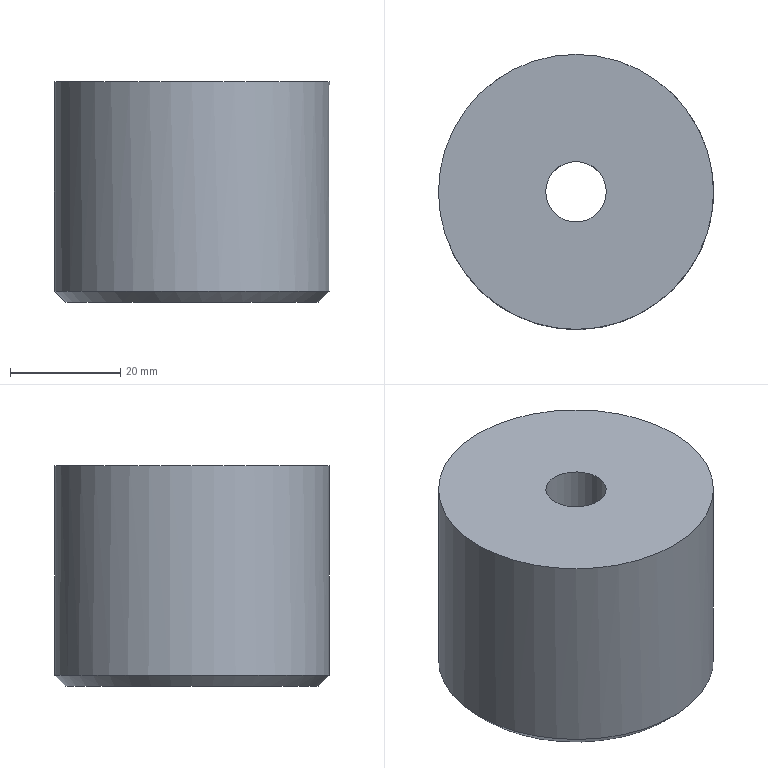Part | STEP file | gslz 2016.10.28-10_id2458_x_t | 1 solid | 7 faces | box 50 x 50 x 40 mm | volume 71266 mm3 | plane 3 | cylinder 3 | cone 1 | commonest cylinder face diameters 11 x1 17 x1 50 x1
STEP:
#1=CARTESIAN_POINT('',(0.,0.,0.));
#2=DIRECTION('',(0.,0.,1.));
#3=DIRECTION('',(1.,0.,0.));
#4=AXIS2_PLACEMENT_3D('',#1,#2,#3);
#5=CARTESIAN_POINT('',(734.,-225.,105.));
#6=VERTEX_POINT('',#5);
#7=CARTESIAN_POINT('',(723.,-225.,105.));
#8=VERTEX_POINT('',#7);
#9=CARTESIAN_POINT('',(728.5,-225.,105.));
#10=DIRECTION('',(0.,0.,1.));
#11=DIRECTION('',(1.,0.,0.));
#12=AXIS2_PLACEMENT_3D('',#9,#10,#11);
#13=CIRCLE('',#12,5.5);
#14=CARTESIAN_POINT('',(676.389,263.723,105.));
#15=DIRECTION('',(0.,0.,1.));
#16=DIRECTION('',(-1.,0.,0.));
#17=AXIS2_PLACEMENT_3D('',#14,#15,#16);
#18=PLANE('',#17);
#19=CARTESIAN_POINT('',(-52.111,488.723));
#20=DIRECTION('',(-1.,0.));
#21=AXIS2_PLACEMENT_2D('',#19,#20);
#22=CIRCLE('',#21,5.5);
#23=(GEOMETRIC_REPRESENTATION_CONTEXT(2)PARAMETRIC_REPRESENTATION_CONTEXT()REPRESENTATION_CONTEXT('',''));
#24=DEFINITIONAL_REPRESENTATION('',(#22),#23);
#25=PCURVE('',#18,#24);
#26=CARTESIAN_POINT('',(728.5,-225.,37.));
#27=DIRECTION('',(0.,0.,1.));
#28=DIRECTION('',(-1.,0.,0.));
#29=AXIS2_PLACEMENT_3D('',#26,#27,#28);
#30=CYLINDRICAL_SURFACE('',#29,5.5);
#31=CARTESIAN_POINT('',(3.142,68.));
#32=DIRECTION('',(1.,0.));
#33=VECTOR('',#32,1.);
#34=LINE('',#31,#33);
#35=(GEOMETRIC_REPRESENTATION_CONTEXT(2)PARAMETRIC_REPRESENTATION_CONTEXT()REPRESENTATION_CONTEXT('',''));
#36=DEFINITIONAL_REPRESENTATION('',(#34),#35);
#37=PCURVE('',#30,#36);
#38=SURFACE_CURVE('',#13,(#25,#37),.PCURVE_S1.);
#39=EDGE_CURVE('',#6,#8,#38,.T.);
#40=ORIENTED_EDGE('',*,*,#39,.F.);
#41=CARTESIAN_POINT('',(728.5,-225.,105.));
#42=DIRECTION('',(0.,0.,1.));
#43=DIRECTION('',(1.,0.,0.));
#44=AXIS2_PLACEMENT_3D('',#41,#42,#43);
#45=CIRCLE('',#44,5.5);
#46=CARTESIAN_POINT('',(-52.111,488.723));
#47=DIRECTION('',(-1.,0.));
#48=AXIS2_PLACEMENT_2D('',#46,#47);
#49=CIRCLE('',#48,5.5);
#50=(GEOMETRIC_REPRESENTATION_CONTEXT(2)PARAMETRIC_REPRESENTATION_CONTEXT()REPRESENTATION_CONTEXT('',''));
#51=DEFINITIONAL_REPRESENTATION('',(#49),#50);
#52=PCURVE('',#18,#51);
#53=CARTESIAN_POINT('',(-3.142,68.));
#54=DIRECTION('',(1.,0.));
#55=VECTOR('',#54,1.);
#56=LINE('',#53,#55);
#57=(GEOMETRIC_REPRESENTATION_CONTEXT(2)PARAMETRIC_REPRESENTATION_CONTEXT()REPRESENTATION_CONTEXT('',''));
#58=DEFINITIONAL_REPRESENTATION('',(#56),#57);
#59=PCURVE('',#30,#58);
#60=SURFACE_CURVE('',#45,(#52,#59),.PCURVE_S1.);
#61=EDGE_CURVE('',#8,#6,#60,.T.);
#62=ORIENTED_EDGE('',*,*,#61,.F.);
#63=EDGE_LOOP('',(#40,#62));
#64=FACE_BOUND('',#63,.T.);
#65=CARTESIAN_POINT('',(753.5,-225.,105.));
#66=VERTEX_POINT('',#65);
#67=CARTESIAN_POINT('',(703.5,-225.,105.));
#68=VERTEX_POINT('',#67);
#69=CARTESIAN_POINT('',(728.5,-225.,105.));
#70=DIRECTION('',(0.,0.,1.));
#71=DIRECTION('',(1.,0.,0.));
#72=AXIS2_PLACEMENT_3D('',#69,#70,#71);
#73=CIRCLE('',#72,25.);
#74=CARTESIAN_POINT('',(-52.111,488.723));
#75=DIRECTION('',(-1.,0.));
#76=AXIS2_PLACEMENT_2D('',#74,#75);
#77=CIRCLE('',#76,25.);
#78=(GEOMETRIC_REPRESENTATION_CONTEXT(2)PARAMETRIC_REPRESENTATION_CONTEXT()REPRESENTATION_CONTEXT('',''));
#79=DEFINITIONAL_REPRESENTATION('',(#77),#78);
#80=PCURVE('',#18,#79);
#81=CARTESIAN_POINT('',(728.5,-225.,60.));
#82=DIRECTION('',(0.,0.,1.));
#83=DIRECTION('',(-1.,0.,0.));
#84=AXIS2_PLACEMENT_3D('',#81,#82,#83);
#85=CYLINDRICAL_SURFACE('',#84,25.);
#86=CARTESIAN_POINT('',(3.142,45.));
#87=DIRECTION('',(1.,0.));
#88=VECTOR('',#87,1.);
#89=LINE('',#86,#88);
#90=(GEOMETRIC_REPRESENTATION_CONTEXT(2)PARAMETRIC_REPRESENTATION_CONTEXT()REPRESENTATION_CONTEXT('',''));
#91=DEFINITIONAL_REPRESENTATION('',(#89),#90);
#92=PCURVE('',#85,#91);
#93=SURFACE_CURVE('',#73,(#80,#92),.PCURVE_S1.);
#94=EDGE_CURVE('',#66,#68,#93,.T.);
#95=ORIENTED_EDGE('',*,*,#94,.T.);
#96=CARTESIAN_POINT('',(728.5,-225.,105.));
#97=DIRECTION('',(0.,0.,1.));
#98=DIRECTION('',(1.,0.,0.));
#99=AXIS2_PLACEMENT_3D('',#96,#97,#98);
#100=CIRCLE('',#99,25.);
#101=CARTESIAN_POINT('',(-52.111,488.723));
#102=DIRECTION('',(-1.,0.));
#103=AXIS2_PLACEMENT_2D('',#101,#102);
#104=CIRCLE('',#103,25.);
#105=(GEOMETRIC_REPRESENTATION_CONTEXT(2)PARAMETRIC_REPRESENTATION_CONTEXT()REPRESENTATION_CONTEXT('',''));
#106=DEFINITIONAL_REPRESENTATION('',(#104),#105);
#107=PCURVE('',#18,#106);
#108=CARTESIAN_POINT('',(-3.142,45.));
#109=DIRECTION('',(1.,0.));
#110=VECTOR('',#109,1.);
#111=LINE('',#108,#110);
#112=(GEOMETRIC_REPRESENTATION_CONTEXT(2)PARAMETRIC_REPRESENTATION_CONTEXT()REPRESENTATION_CONTEXT('',''));
#113=DEFINITIONAL_REPRESENTATION('',(#111),#112);
#114=PCURVE('',#85,#113);
#115=SURFACE_CURVE('',#100,(#107,#114),.PCURVE_S1.);
#116=EDGE_CURVE('',#68,#66,#115,.T.);
#117=ORIENTED_EDGE('',*,*,#116,.T.);
#118=EDGE_LOOP('',(#95,#117));
#119=FACE_BOUND('',#118,.T.);
#120=ADVANCED_FACE('',(#64,#119),#18,.T.);
#121=CARTESIAN_POINT('',(705.5,-225.,65.));
#122=VERTEX_POINT('',#121);
#123=CARTESIAN_POINT('',(728.5,-225.,65.));
#124=DIRECTION('',(0.,0.,-1.));
#125=DIRECTION('',(-1.,0.,0.));
#126=AXIS2_PLACEMENT_3D('',#123,#124,#125);
#127=CIRCLE('',#126,23.);
#128=CARTESIAN_POINT('',(728.5,-225.,65.));
#129=DIRECTION('',(0.,0.,-1.));
#130=DIRECTION('',(1.,0.,0.));
#131=AXIS2_PLACEMENT_3D('',#128,#129,#130);
#132=PLANE('',#131);
#133=CARTESIAN_POINT('',(0.,0.));
#134=DIRECTION('',(-1.,0.));
#135=AXIS2_PLACEMENT_2D('',#133,#134);
#136=CIRCLE('',#135,23.);
#137=(GEOMETRIC_REPRESENTATION_CONTEXT(2)PARAMETRIC_REPRESENTATION_CONTEXT()REPRESENTATION_CONTEXT('',''));
#138=DEFINITIONAL_REPRESENTATION('',(#136),#137);
#139=PCURVE('',#132,#138);
#140=CARTESIAN_POINT('',(728.5,-225.,65.));
#141=DIRECTION('',(0.,0.,1.));
#142=DIRECTION('',(-1.,0.,0.));
#143=AXIS2_PLACEMENT_3D('',#140,#141,#142);
#144=CONICAL_SURFACE('',#143,23.,0.7854);
#145=CARTESIAN_POINT('',(6.283,0.));
#146=DIRECTION('',(-1.,0.));
#147=VECTOR('',#146,1.);
#148=LINE('',#145,#147);
#149=(GEOMETRIC_REPRESENTATION_CONTEXT(2)PARAMETRIC_REPRESENTATION_CONTEXT()REPRESENTATION_CONTEXT('',''));
#150=DEFINITIONAL_REPRESENTATION('',(#148),#149);
#151=PCURVE('',#144,#150);
#152=SURFACE_CURVE('',#127,(#139,#151),.PCURVE_S1.);
#153=EDGE_CURVE('',#122,#122,#152,.T.);
#154=ORIENTED_EDGE('',*,*,#153,.T.);
#155=EDGE_LOOP('',(#154));
#156=FACE_BOUND('',#155,.T.);
#157=CARTESIAN_POINT('',(720.,-225.,65.));
#158=VERTEX_POINT('',#157);
#159=CARTESIAN_POINT('',(728.5,-225.,65.));
#160=DIRECTION('',(0.,0.,1.));
#161=DIRECTION('',(-1.,0.,0.));
#162=AXIS2_PLACEMENT_3D('',#159,#160,#161);
#163=CIRCLE('',#162,8.5);
#164=CARTESIAN_POINT('',(-8.5,0.));
#165=CARTESIAN_POINT('',(-8.5,14.722));
#166=CARTESIAN_POINT('',(4.25,7.361));
#167=CARTESIAN_POINT('',(17.,0.));
#168=CARTESIAN_POINT('',(4.25,-7.361));
#169=CARTESIAN_POINT('',(-8.5,-14.722));
#170=CARTESIAN_POINT('',(-8.5,0.));
#171=(BOUNDED_CURVE()B_SPLINE_CURVE(2,(#164,#165,#166,#167,#168,#169,#170),.UNSPECIFIED.,.T.,.F.)B_SPLINE_CURVE_WITH_KNOTS((1,2,2,2,2,1),(-2.094,0.,2.094,4.189,6.283,8.378),.UNSPECIFIED.)CURVE()GEOMETRIC_REPRESENTATION_ITEM()RATIONAL_B_SPLINE_CURVE((1.,0.5,1.,0.5,1.,0.5,1.))REPRESENTATION_ITEM(''));
#172=(GEOMETRIC_REPRESENTATION_CONTEXT(2)PARAMETRIC_REPRESENTATION_CONTEXT()REPRESENTATION_CONTEXT('',''));
#173=DEFINITIONAL_REPRESENTATION('',(#171),#172);
#174=PCURVE('',#132,#173);
#175=CARTESIAN_POINT('',(728.5,-225.,65.));
#176=DIRECTION('',(0.,0.,1.));
#177=DIRECTION('',(-1.,0.,0.));
#178=AXIS2_PLACEMENT_3D('',#175,#176,#177);
#179=CYLINDRICAL_SURFACE('',#178,8.5);
#180=CARTESIAN_POINT('',(0.,0.));
#181=DIRECTION('',(1.,0.));
#182=VECTOR('',#181,1.);
#183=LINE('',#180,#182);
#184=(GEOMETRIC_REPRESENTATION_CONTEXT(2)PARAMETRIC_REPRESENTATION_CONTEXT()REPRESENTATION_CONTEXT('',''));
#185=DEFINITIONAL_REPRESENTATION('',(#183),#184);
#186=PCURVE('',#179,#185);
#187=SURFACE_CURVE('',#163,(#174,#186),.PCURVE_S1.);
#188=EDGE_CURVE('',#158,#158,#187,.T.);
#189=ORIENTED_EDGE('',*,*,#188,.T.);
#190=EDGE_LOOP('',(#189));
#191=FACE_BOUND('',#190,.T.);
#192=ADVANCED_FACE('',(#156,#191),#132,.T.);
#193=ORIENTED_EDGE('',*,*,#116,.F.);
#194=CARTESIAN_POINT('',(703.5,-225.,67.));
#195=VERTEX_POINT('',#194);
#196=CARTESIAN_POINT('',(703.5,-225.,67.));
#197=CARTESIAN_POINT('',(703.5,-225.,105.));
#198=B_SPLINE_CURVE_WITH_KNOTS('',1,(#196,#197),.UNSPECIFIED.,.F.,.F.,(2,2),(7.,45.),.PIECEWISE_BEZIER_KNOTS.);
#199=CARTESIAN_POINT('',(0.,0.));
#200=DIRECTION('',(0.,1.));
#201=VECTOR('',#200,1.);
#202=LINE('',#199,#201);
#203=(GEOMETRIC_REPRESENTATION_CONTEXT(2)PARAMETRIC_REPRESENTATION_CONTEXT()REPRESENTATION_CONTEXT('',''));
#204=DEFINITIONAL_REPRESENTATION('',(#202),#203);
#205=PCURVE('',#85,#204);
#206=CARTESIAN_POINT('',(6.283,0.));
#207=DIRECTION('',(0.,1.));
#208=VECTOR('',#207,1.);
#209=LINE('',#206,#208);
#210=(GEOMETRIC_REPRESENTATION_CONTEXT(2)PARAMETRIC_REPRESENTATION_CONTEXT()REPRESENTATION_CONTEXT('',''));
#211=DEFINITIONAL_REPRESENTATION('',(#209),#210);
#212=PCURVE('',#85,#211);
#213=SEAM_CURVE('',#198,(#205,#212),.PCURVE_S1.);
#214=EDGE_CURVE('',#195,#68,#213,.T.);
#215=ORIENTED_EDGE('',*,*,#214,.F.);
#216=CARTESIAN_POINT('',(728.5,-225.,67.));
#217=DIRECTION('',(0.,0.,1.));
#218=DIRECTION('',(-1.,0.,0.));
#219=AXIS2_PLACEMENT_3D('',#216,#217,#218);
#220=CIRCLE('',#219,25.);
#221=CARTESIAN_POINT('',(0.,7.));
#222=DIRECTION('',(1.,0.));
#223=VECTOR('',#222,1.);
#224=LINE('',#221,#223);
#225=(GEOMETRIC_REPRESENTATION_CONTEXT(2)PARAMETRIC_REPRESENTATION_CONTEXT()REPRESENTATION_CONTEXT('',''));
#226=DEFINITIONAL_REPRESENTATION('',(#224),#225);
#227=PCURVE('',#85,#226);
#228=CARTESIAN_POINT('',(0.,2.));
#229=DIRECTION('',(1.,0.));
#230=VECTOR('',#229,1.);
#231=LINE('',#228,#230);
#232=(GEOMETRIC_REPRESENTATION_CONTEXT(2)PARAMETRIC_REPRESENTATION_CONTEXT()REPRESENTATION_CONTEXT('',''));
#233=DEFINITIONAL_REPRESENTATION('',(#231),#232);
#234=PCURVE('',#144,#233);
#235=SURFACE_CURVE('',#220,(#227,#234),.PCURVE_S1.);
#236=EDGE_CURVE('',#195,#195,#235,.T.);
#237=ORIENTED_EDGE('',*,*,#236,.T.);
#238=ORIENTED_EDGE('',*,*,#214,.T.);
#239=ORIENTED_EDGE('',*,*,#94,.F.);
#240=EDGE_LOOP('',(#193,#215,#237,#238,#239));
#241=FACE_BOUND('',#240,.T.);
#242=ADVANCED_FACE('',(#241),#85,.T.);
#243=ORIENTED_EDGE('',*,*,#61,.F.);
#244=CARTESIAN_POINT('',(723.,-225.,89.));
#245=VERTEX_POINT('',#244);
#246=CARTESIAN_POINT('',(723.,-225.,89.));
#247=CARTESIAN_POINT('',(723.,-225.,105.));
#248=B_SPLINE_CURVE_WITH_KNOTS('',1,(#246,#247),.UNSPECIFIED.,.F.,.F.,(2,2),(52.,68.),.PIECEWISE_BEZIER_KNOTS.);
#249=CARTESIAN_POINT('',(0.,0.));
#250=DIRECTION('',(0.,1.));
#251=VECTOR('',#250,1.);
#252=LINE('',#249,#251);
#253=(GEOMETRIC_REPRESENTATION_CONTEXT(2)PARAMETRIC_REPRESENTATION_CONTEXT()REPRESENTATION_CONTEXT('',''));
#254=DEFINITIONAL_REPRESENTATION('',(#252),#253);
#255=PCURVE('',#30,#254);
#256=CARTESIAN_POINT('',(6.283,0.));
#257=DIRECTION('',(0.,1.));
#258=VECTOR('',#257,1.);
#259=LINE('',#256,#258);
#260=(GEOMETRIC_REPRESENTATION_CONTEXT(2)PARAMETRIC_REPRESENTATION_CONTEXT()REPRESENTATION_CONTEXT('',''));
#261=DEFINITIONAL_REPRESENTATION('',(#259),#260);
#262=PCURVE('',#30,#261);
#263=SEAM_CURVE('',#248,(#255,#262),.PCURVE_S1.);
#264=EDGE_CURVE('',#245,#8,#263,.T.);
#265=ORIENTED_EDGE('',*,*,#264,.F.);
#266=CARTESIAN_POINT('',(728.5,-225.,89.));
#267=DIRECTION('',(0.,0.,-1.));
#268=DIRECTION('',(-1.,0.,0.));
#269=AXIS2_PLACEMENT_3D('',#266,#267,#268);
#270=CIRCLE('',#269,5.5);
#271=CARTESIAN_POINT('',(6.283,52.));
#272=DIRECTION('',(-1.,0.));
#273=VECTOR('',#272,1.);
#274=LINE('',#271,#273);
#275=(GEOMETRIC_REPRESENTATION_CONTEXT(2)PARAMETRIC_REPRESENTATION_CONTEXT()REPRESENTATION_CONTEXT('',''));
#276=DEFINITIONAL_REPRESENTATION('',(#274),#275);
#277=PCURVE('',#30,#276);
#278=CARTESIAN_POINT('',(728.5,-225.,89.));
#279=DIRECTION('',(0.,0.,-1.));
#280=DIRECTION('',(1.,0.,0.));
#281=AXIS2_PLACEMENT_3D('',#278,#279,#280);
#282=PLANE('',#281);
#283=CARTESIAN_POINT('',(0.,0.));
#284=DIRECTION('',(-1.,0.));
#285=AXIS2_PLACEMENT_2D('',#283,#284);
#286=CIRCLE('',#285,5.5);
#287=(GEOMETRIC_REPRESENTATION_CONTEXT(2)PARAMETRIC_REPRESENTATION_CONTEXT()REPRESENTATION_CONTEXT('',''));
#288=DEFINITIONAL_REPRESENTATION('',(#286),#287);
#289=PCURVE('',#282,#288);
#290=SURFACE_CURVE('',#270,(#277,#289),.PCURVE_S1.);
#291=EDGE_CURVE('',#245,#245,#290,.T.);
#292=ORIENTED_EDGE('',*,*,#291,.F.);
#293=ORIENTED_EDGE('',*,*,#264,.T.);
#294=ORIENTED_EDGE('',*,*,#39,.F.);
#295=EDGE_LOOP('',(#243,#265,#292,#293,#294));
#296=FACE_BOUND('',#295,.F.);
#297=ADVANCED_FACE('',(#296),#30,.F.);
#298=CARTESIAN_POINT('',(720.,-225.,89.));
#299=VERTEX_POINT('',#298);
#300=CARTESIAN_POINT('',(728.5,-225.,89.));
#301=DIRECTION('',(0.,0.,-1.));
#302=DIRECTION('',(-1.,0.,0.));
#303=AXIS2_PLACEMENT_3D('',#300,#301,#302);
#304=CIRCLE('',#303,8.5);
#305=CARTESIAN_POINT('',(0.,0.));
#306=DIRECTION('',(-1.,0.));
#307=AXIS2_PLACEMENT_2D('',#305,#306);
#308=CIRCLE('',#307,8.5);
#309=(GEOMETRIC_REPRESENTATION_CONTEXT(2)PARAMETRIC_REPRESENTATION_CONTEXT()REPRESENTATION_CONTEXT('',''));
#310=DEFINITIONAL_REPRESENTATION('',(#308),#309);
#311=PCURVE('',#282,#310);
#312=CARTESIAN_POINT('',(6.283,24.));
#313=DIRECTION('',(-1.,0.));
#314=VECTOR('',#313,1.);
#315=LINE('',#312,#314);
#316=(GEOMETRIC_REPRESENTATION_CONTEXT(2)PARAMETRIC_REPRESENTATION_CONTEXT()REPRESENTATION_CONTEXT('',''));
#317=DEFINITIONAL_REPRESENTATION('',(#315),#316);
#318=PCURVE('',#179,#317);
#319=SURFACE_CURVE('',#304,(#311,#318),.PCURVE_S1.);
#320=EDGE_CURVE('',#299,#299,#319,.T.);
#321=ORIENTED_EDGE('',*,*,#320,.T.);
#322=EDGE_LOOP('',(#321));
#323=FACE_BOUND('',#322,.T.);
#324=ORIENTED_EDGE('',*,*,#291,.F.);
#325=EDGE_LOOP('',(#324));
#326=FACE_BOUND('',#325,.T.);
#327=ADVANCED_FACE('',(#323,#326),#282,.T.);
#328=ORIENTED_EDGE('',*,*,#188,.T.);
#329=CARTESIAN_POINT('',(720.,-225.,65.));
#330=CARTESIAN_POINT('',(720.,-225.,89.));
#331=B_SPLINE_CURVE_WITH_KNOTS('',1,(#329,#330),.UNSPECIFIED.,.F.,.F.,(2,2),(0.,24.),.PIECEWISE_BEZIER_KNOTS.);
#332=CARTESIAN_POINT('',(6.283,0.));
#333=DIRECTION('',(0.,1.));
#334=VECTOR('',#333,1.);
#335=LINE('',#332,#334);
#336=(GEOMETRIC_REPRESENTATION_CONTEXT(2)PARAMETRIC_REPRESENTATION_CONTEXT()REPRESENTATION_CONTEXT('',''));
#337=DEFINITIONAL_REPRESENTATION('',(#335),#336);
#338=PCURVE('',#179,#337);
#339=CARTESIAN_POINT('',(0.,0.));
#340=DIRECTION('',(0.,1.));
#341=VECTOR('',#340,1.);
#342=LINE('',#339,#341);
#343=(GEOMETRIC_REPRESENTATION_CONTEXT(2)PARAMETRIC_REPRESENTATION_CONTEXT()REPRESENTATION_CONTEXT('',''));
#344=DEFINITIONAL_REPRESENTATION('',(#342),#343);
#345=PCURVE('',#179,#344);
#346=SEAM_CURVE('',#331,(#338,#345),.PCURVE_S1.);
#347=EDGE_CURVE('',#158,#299,#346,.T.);
#348=ORIENTED_EDGE('',*,*,#347,.T.);
#349=ORIENTED_EDGE('',*,*,#320,.T.);
#350=ORIENTED_EDGE('',*,*,#347,.F.);
#351=EDGE_LOOP('',(#328,#348,#349,#350));
#352=FACE_BOUND('',#351,.F.);
#353=ADVANCED_FACE('',(#352),#179,.F.);
#354=ORIENTED_EDGE('',*,*,#236,.F.);
#355=CARTESIAN_POINT('',(705.5,-225.,65.));
#356=CARTESIAN_POINT('',(703.5,-225.,67.));
#357=B_SPLINE_CURVE_WITH_KNOTS('',1,(#355,#356),.UNSPECIFIED.,.F.,.F.,(2,2),(0.,2.828),.PIECEWISE_BEZIER_KNOTS.);
#358=CARTESIAN_POINT('',(0.,0.));
#359=DIRECTION('',(0.,1.));
#360=VECTOR('',#359,1.);
#361=LINE('',#358,#360);
#362=(GEOMETRIC_REPRESENTATION_CONTEXT(2)PARAMETRIC_REPRESENTATION_CONTEXT()REPRESENTATION_CONTEXT('',''));
#363=DEFINITIONAL_REPRESENTATION('',(#361),#362);
#364=PCURVE('',#144,#363);
#365=CARTESIAN_POINT('',(6.283,0.));
#366=DIRECTION('',(0.,1.));
#367=VECTOR('',#366,1.);
#368=LINE('',#365,#367);
#369=(GEOMETRIC_REPRESENTATION_CONTEXT(2)PARAMETRIC_REPRESENTATION_CONTEXT()REPRESENTATION_CONTEXT('',''));
#370=DEFINITIONAL_REPRESENTATION('',(#368),#369);
#371=PCURVE('',#144,#370);
#372=SEAM_CURVE('',#357,(#364,#371),.PCURVE_S1.);
#373=EDGE_CURVE('',#122,#195,#372,.T.);
#374=ORIENTED_EDGE('',*,*,#373,.F.);
#375=ORIENTED_EDGE('',*,*,#153,.F.);
#376=ORIENTED_EDGE('',*,*,#373,.T.);
#377=EDGE_LOOP('',(#354,#374,#375,#376));
#378=FACE_BOUND('',#377,.T.);
#379=ADVANCED_FACE('',(#378),#144,.T.);
#380=CLOSED_SHELL('',(#120,#192,#242,#297,#327,#353,#379));
#381=MANIFOLD_SOLID_BREP('',#380);
#382=(LENGTH_UNIT()NAMED_UNIT(*)SI_UNIT(.MILLI.,.METRE.));
#383=UNCERTAINTY_MEASURE_WITH_UNIT(LENGTH_MEASURE(0.000005),#382,'','');
#384=(NAMED_UNIT(*)PLANE_ANGLE_UNIT()SI_UNIT($,.RADIAN.));
#385=(NAMED_UNIT(*)SI_UNIT($,.STERADIAN.)SOLID_ANGLE_UNIT());
#386=(GEOMETRIC_REPRESENTATION_CONTEXT(3)GLOBAL_UNCERTAINTY_ASSIGNED_CONTEXT((#383))GLOBAL_UNIT_ASSIGNED_CONTEXT((#382,#384,#385))REPRESENTATION_CONTEXT('',''));
#387=ADVANCED_BREP_SHAPE_REPRESENTATION('',(#4,#381),#386);